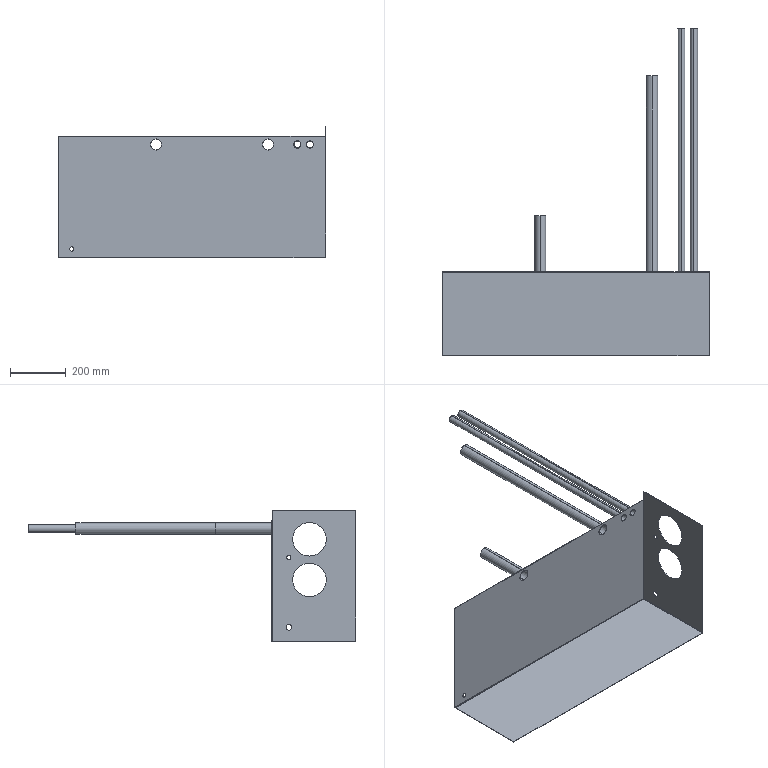Part | 2 solids | 55 faces | box 956 x 1170 x 470 mm | volume 1222828 mm3 | cylinder 32 | plane 21 | spline 2 | commonest cylinder face diameters 38 x6 15 x4 24 x4 26 x4 40 x4 120 x4